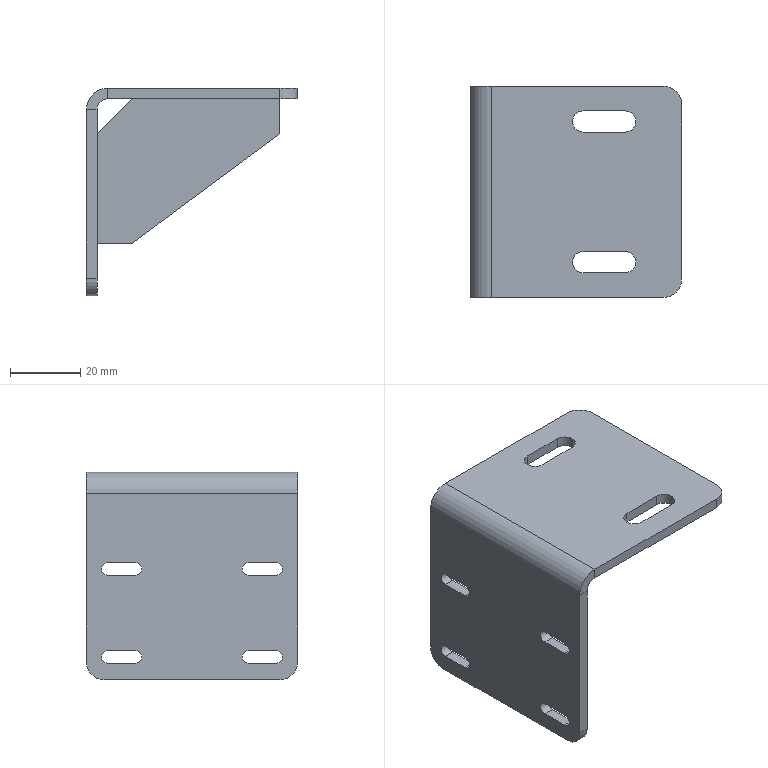Part | STEP file | Drive module fixing part V1.201001 | 2 solids | 52 faces | box 60 x 60 x 59 mm | volume 23708 mm3 | plane 32 | cylinder 20 | commonest cylinder face diameters 3.5 x8 6 x7 10 x4 12 x1